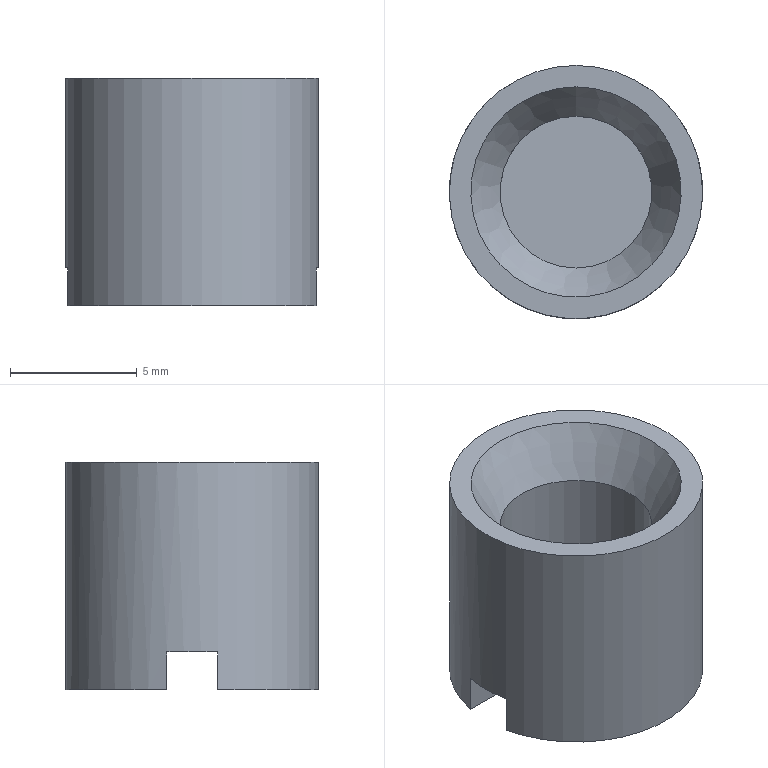Part | STEP file | 1-67.4 | 1 solid | 10 faces | box 10 x 10 x 9 mm | volume 482.855 mm3 | plane 7 | cylinder 2 | cone 1 | commonest cylinder face diameters 6 x1 10 x1
STEP:
#1=CARTESIAN_POINT('',(0.,0.,0.));
#2=DIRECTION('',(0.,0.,1.));
#3=DIRECTION('',(1.,0.,0.));
#4=AXIS2_PLACEMENT_3D('',#1,#2,#3);
#5=CARTESIAN_POINT('',(0.,5.,0.));
#6=VERTEX_POINT('',#5);
#7=CARTESIAN_POINT('',(-4.899,1.,0.));
#8=VERTEX_POINT('',#7);
#9=CARTESIAN_POINT('',(0.,0.,0.));
#10=DIRECTION('',(0.,0.,1.));
#11=DIRECTION('',(0.,1.,0.));
#12=AXIS2_PLACEMENT_3D('',#9,#10,#11);
#13=CIRCLE('',#12,5.);
#14=CARTESIAN_POINT('',(0.,-2.5,0.));
#15=DIRECTION('',(0.,0.,1.));
#16=DIRECTION('',(0.,1.,0.));
#17=AXIS2_PLACEMENT_3D('',#14,#15,#16);
#18=PLANE('',#17);
#19=CARTESIAN_POINT('',(2.5,0.));
#20=DIRECTION('',(1.,0.));
#21=AXIS2_PLACEMENT_2D('',#19,#20);
#22=CIRCLE('',#21,5.);
#23=(GEOMETRIC_REPRESENTATION_CONTEXT(2)PARAMETRIC_REPRESENTATION_CONTEXT()REPRESENTATION_CONTEXT('',''));
#24=DEFINITIONAL_REPRESENTATION('',(#22),#23);
#25=PCURVE('',#18,#24);
#26=CARTESIAN_POINT('',(0.,0.,0.));
#27=DIRECTION('',(0.,0.,1.));
#28=DIRECTION('',(0.,1.,0.));
#29=AXIS2_PLACEMENT_3D('',#26,#27,#28);
#30=CYLINDRICAL_SURFACE('',#29,5.);
#31=CARTESIAN_POINT('',(0.,0.));
#32=DIRECTION('',(1.,0.));
#33=VECTOR('',#32,1.);
#34=LINE('',#31,#33);
#35=(GEOMETRIC_REPRESENTATION_CONTEXT(2)PARAMETRIC_REPRESENTATION_CONTEXT()REPRESENTATION_CONTEXT('',''));
#36=DEFINITIONAL_REPRESENTATION('',(#34),#35);
#37=PCURVE('',#30,#36);
#38=SURFACE_CURVE('',#13,(#25,#37),.PCURVE_S1.);
#39=EDGE_CURVE('',#6,#8,#38,.T.);
#40=ORIENTED_EDGE('',*,*,#39,.T.);
#41=CARTESIAN_POINT('',(4.899,1.,0.));
#42=VERTEX_POINT('',#41);
#43=CARTESIAN_POINT('',(-4.899,1.,0.));
#44=DIRECTION('',(1.,0.,0.));
#45=VECTOR('',#44,1.);
#46=LINE('',#43,#45);
#47=CARTESIAN_POINT('',(3.5,4.899));
#48=DIRECTION('',(0.,-1.));
#49=VECTOR('',#48,1.);
#50=LINE('',#47,#49);
#51=(GEOMETRIC_REPRESENTATION_CONTEXT(2)PARAMETRIC_REPRESENTATION_CONTEXT()REPRESENTATION_CONTEXT('',''));
#52=DEFINITIONAL_REPRESENTATION('',(#50),#51);
#53=PCURVE('',#18,#52);
#54=CARTESIAN_POINT('',(0.,1.,0.));
#55=DIRECTION('',(0.,1.,0.));
#56=DIRECTION('',(0.,0.,1.));
#57=AXIS2_PLACEMENT_3D('',#54,#55,#56);
#58=PLANE('',#57);
#59=CARTESIAN_POINT('',(0.,-4.899));
#60=DIRECTION('',(0.,1.));
#61=VECTOR('',#60,1.);
#62=LINE('',#59,#61);
#63=(GEOMETRIC_REPRESENTATION_CONTEXT(2)PARAMETRIC_REPRESENTATION_CONTEXT()REPRESENTATION_CONTEXT('',''));
#64=DEFINITIONAL_REPRESENTATION('',(#62),#63);
#65=PCURVE('',#58,#64);
#66=SURFACE_CURVE('',#46,(#53,#65),.PCURVE_S1.);
#67=EDGE_CURVE('',#8,#42,#66,.T.);
#68=ORIENTED_EDGE('',*,*,#67,.T.);
#69=CARTESIAN_POINT('',(0.,0.,0.));
#70=DIRECTION('',(0.,0.,1.));
#71=DIRECTION('',(0.9798,0.2,0.));
#72=AXIS2_PLACEMENT_3D('',#69,#70,#71);
#73=CIRCLE('',#72,5.);
#74=CARTESIAN_POINT('',(2.5,0.));
#75=DIRECTION('',(0.2,-0.9798));
#76=AXIS2_PLACEMENT_2D('',#74,#75);
#77=CIRCLE('',#76,5.);
#78=(GEOMETRIC_REPRESENTATION_CONTEXT(2)PARAMETRIC_REPRESENTATION_CONTEXT()REPRESENTATION_CONTEXT('',''));
#79=DEFINITIONAL_REPRESENTATION('',(#77),#78);
#80=PCURVE('',#18,#79);
#81=CARTESIAN_POINT('',(4.914,0.));
#82=DIRECTION('',(1.,0.));
#83=VECTOR('',#82,1.);
#84=LINE('',#81,#83);
#85=(GEOMETRIC_REPRESENTATION_CONTEXT(2)PARAMETRIC_REPRESENTATION_CONTEXT()REPRESENTATION_CONTEXT('',''));
#86=DEFINITIONAL_REPRESENTATION('',(#84),#85);
#87=PCURVE('',#30,#86);
#88=SURFACE_CURVE('',#73,(#80,#87),.PCURVE_S1.);
#89=EDGE_CURVE('',#42,#6,#88,.T.);
#90=ORIENTED_EDGE('',*,*,#89,.T.);
#91=EDGE_LOOP('',(#40,#68,#90));
#92=FACE_BOUND('',#91,.F.);
#93=ADVANCED_FACE('',(#92),#18,.F.);
#94=CARTESIAN_POINT('',(-4.899,-1.,0.));
#95=VERTEX_POINT('',#94);
#96=CARTESIAN_POINT('',(4.899,-1.,0.));
#97=VERTEX_POINT('',#96);
#98=CARTESIAN_POINT('',(0.,0.,0.));
#99=DIRECTION('',(0.,0.,1.));
#100=DIRECTION('',(-0.9798,-0.2,0.));
#101=AXIS2_PLACEMENT_3D('',#98,#99,#100);
#102=CIRCLE('',#101,5.);
#103=CARTESIAN_POINT('',(0.,-2.5,0.));
#104=DIRECTION('',(0.,0.,1.));
#105=DIRECTION('',(0.,1.,0.));
#106=AXIS2_PLACEMENT_3D('',#103,#104,#105);
#107=PLANE('',#106);
#108=CARTESIAN_POINT('',(2.5,0.));
#109=DIRECTION('',(-0.2,0.9798));
#110=AXIS2_PLACEMENT_2D('',#108,#109);
#111=CIRCLE('',#110,5.);
#112=(GEOMETRIC_REPRESENTATION_CONTEXT(2)PARAMETRIC_REPRESENTATION_CONTEXT()REPRESENTATION_CONTEXT('',''));
#113=DEFINITIONAL_REPRESENTATION('',(#111),#112);
#114=PCURVE('',#107,#113);
#115=CARTESIAN_POINT('',(1.772,0.));
#116=DIRECTION('',(1.,0.));
#117=VECTOR('',#116,1.);
#118=LINE('',#115,#117);
#119=(GEOMETRIC_REPRESENTATION_CONTEXT(2)PARAMETRIC_REPRESENTATION_CONTEXT()REPRESENTATION_CONTEXT('',''));
#120=DEFINITIONAL_REPRESENTATION('',(#118),#119);
#121=PCURVE('',#30,#120);
#122=SURFACE_CURVE('',#102,(#114,#121),.PCURVE_S1.);
#123=EDGE_CURVE('',#95,#97,#122,.T.);
#124=ORIENTED_EDGE('',*,*,#123,.T.);
#125=CARTESIAN_POINT('',(4.899,-1.,0.));
#126=DIRECTION('',(-1.,0.,0.));
#127=VECTOR('',#126,1.);
#128=LINE('',#125,#127);
#129=CARTESIAN_POINT('',(1.5,-4.899));
#130=DIRECTION('',(0.,1.));
#131=VECTOR('',#130,1.);
#132=LINE('',#129,#131);
#133=(GEOMETRIC_REPRESENTATION_CONTEXT(2)PARAMETRIC_REPRESENTATION_CONTEXT()REPRESENTATION_CONTEXT('',''));
#134=DEFINITIONAL_REPRESENTATION('',(#132),#133);
#135=PCURVE('',#107,#134);
#136=CARTESIAN_POINT('',(0.,-1.,0.));
#137=DIRECTION('',(0.,-1.,0.));
#138=DIRECTION('',(0.,0.,-1.));
#139=AXIS2_PLACEMENT_3D('',#136,#137,#138);
#140=PLANE('',#139);
#141=CARTESIAN_POINT('',(0.,4.899));
#142=DIRECTION('',(0.,-1.));
#143=VECTOR('',#142,1.);
#144=LINE('',#141,#143);
#145=(GEOMETRIC_REPRESENTATION_CONTEXT(2)PARAMETRIC_REPRESENTATION_CONTEXT()REPRESENTATION_CONTEXT('',''));
#146=DEFINITIONAL_REPRESENTATION('',(#144),#145);
#147=PCURVE('',#140,#146);
#148=SURFACE_CURVE('',#128,(#135,#147),.PCURVE_S1.);
#149=EDGE_CURVE('',#97,#95,#148,.T.);
#150=ORIENTED_EDGE('',*,*,#149,.T.);
#151=EDGE_LOOP('',(#124,#150));
#152=FACE_BOUND('',#151,.F.);
#153=ADVANCED_FACE('',(#152),#107,.F.);
#154=ORIENTED_EDGE('',*,*,#39,.T.);
#155=CARTESIAN_POINT('',(-4.899,1.,1.5));
#156=VERTEX_POINT('',#155);
#157=CARTESIAN_POINT('',(-4.899,1.,1.5));
#158=DIRECTION('',(0.,0.,-1.));
#159=VECTOR('',#158,1.);
#160=LINE('',#157,#159);
#161=CARTESIAN_POINT('',(1.369,1.5));
#162=DIRECTION('',(0.,-1.));
#163=VECTOR('',#162,1.);
#164=LINE('',#161,#163);
#165=(GEOMETRIC_REPRESENTATION_CONTEXT(2)PARAMETRIC_REPRESENTATION_CONTEXT()REPRESENTATION_CONTEXT('',''));
#166=DEFINITIONAL_REPRESENTATION('',(#164),#165);
#167=PCURVE('',#30,#166);
#168=CARTESIAN_POINT('',(1.5,-4.899));
#169=DIRECTION('',(-1.,0.));
#170=VECTOR('',#169,1.);
#171=LINE('',#168,#170);
#172=(GEOMETRIC_REPRESENTATION_CONTEXT(2)PARAMETRIC_REPRESENTATION_CONTEXT()REPRESENTATION_CONTEXT('',''));
#173=DEFINITIONAL_REPRESENTATION('',(#171),#172);
#174=PCURVE('',#58,#173);
#175=SURFACE_CURVE('',#160,(#167,#174),.PCURVE_S1.);
#176=EDGE_CURVE('',#156,#8,#175,.T.);
#177=ORIENTED_EDGE('',*,*,#176,.F.);
#178=CARTESIAN_POINT('',(-4.899,-1.,1.5));
#179=VERTEX_POINT('',#178);
#180=CARTESIAN_POINT('',(0.,0.,1.5));
#181=DIRECTION('',(0.,0.,-1.));
#182=DIRECTION('',(-0.9798,-0.2,0.));
#183=AXIS2_PLACEMENT_3D('',#180,#181,#182);
#184=CIRCLE('',#183,5.);
#185=CARTESIAN_POINT('',(1.772,1.5));
#186=DIRECTION('',(-1.,0.));
#187=VECTOR('',#186,1.);
#188=LINE('',#185,#187);
#189=(GEOMETRIC_REPRESENTATION_CONTEXT(2)PARAMETRIC_REPRESENTATION_CONTEXT()REPRESENTATION_CONTEXT('',''));
#190=DEFINITIONAL_REPRESENTATION('',(#188),#189);
#191=PCURVE('',#30,#190);
#192=CARTESIAN_POINT('',(0.,0.,1.5));
#193=DIRECTION('',(0.,0.,1.));
#194=DIRECTION('',(0.,-1.,0.));
#195=AXIS2_PLACEMENT_3D('',#192,#193,#194);
#196=PLANE('',#195);
#197=CARTESIAN_POINT('',(1.,-4.899));
#198=CARTESIAN_POINT('',(-7.485,-6.631));
#199=CARTESIAN_POINT('',(-4.743,1.583));
#200=CARTESIAN_POINT('',(-2.,9.798));
#201=CARTESIAN_POINT('',(3.743,3.316));
#202=CARTESIAN_POINT('',(9.485,-3.167));
#203=CARTESIAN_POINT('',(1.,-4.899));
#204=(BOUNDED_CURVE()B_SPLINE_CURVE(2,(#197,#198,#199,#200,#201,#202,#203),.UNSPECIFIED.,.T.,.F.)B_SPLINE_CURVE_WITH_KNOTS((1,2,2,2,2,1),(-2.094,0.,2.094,4.189,6.283,8.378),.UNSPECIFIED.)CURVE()GEOMETRIC_REPRESENTATION_ITEM()RATIONAL_B_SPLINE_CURVE((1.,0.5,1.,0.5,1.,0.5,1.))REPRESENTATION_ITEM(''));
#205=(GEOMETRIC_REPRESENTATION_CONTEXT(2)PARAMETRIC_REPRESENTATION_CONTEXT()REPRESENTATION_CONTEXT('',''));
#206=DEFINITIONAL_REPRESENTATION('',(#204),#205);
#207=PCURVE('',#196,#206);
#208=SURFACE_CURVE('',#184,(#191,#207),.PCURVE_S1.);
#209=EDGE_CURVE('',#179,#156,#208,.T.);
#210=ORIENTED_EDGE('',*,*,#209,.F.);
#211=CARTESIAN_POINT('',(-4.899,-1.,0.));
#212=DIRECTION('',(0.,0.,1.));
#213=VECTOR('',#212,1.);
#214=LINE('',#211,#213);
#215=CARTESIAN_POINT('',(1.772,0.));
#216=DIRECTION('',(0.,1.));
#217=VECTOR('',#216,1.);
#218=LINE('',#215,#217);
#219=(GEOMETRIC_REPRESENTATION_CONTEXT(2)PARAMETRIC_REPRESENTATION_CONTEXT()REPRESENTATION_CONTEXT('',''));
#220=DEFINITIONAL_REPRESENTATION('',(#218),#219);
#221=PCURVE('',#30,#220);
#222=CARTESIAN_POINT('',(0.,-4.899));
#223=DIRECTION('',(-1.,0.));
#224=VECTOR('',#223,1.);
#225=LINE('',#222,#224);
#226=(GEOMETRIC_REPRESENTATION_CONTEXT(2)PARAMETRIC_REPRESENTATION_CONTEXT()REPRESENTATION_CONTEXT('',''));
#227=DEFINITIONAL_REPRESENTATION('',(#225),#226);
#228=PCURVE('',#140,#227);
#229=SURFACE_CURVE('',#214,(#221,#228),.PCURVE_S1.);
#230=EDGE_CURVE('',#95,#179,#229,.T.);
#231=ORIENTED_EDGE('',*,*,#230,.F.);
#232=ORIENTED_EDGE('',*,*,#123,.T.);
#233=CARTESIAN_POINT('',(4.899,-1.,1.5));
#234=VERTEX_POINT('',#233);
#235=CARTESIAN_POINT('',(4.899,-1.,1.5));
#236=DIRECTION('',(0.,0.,-1.));
#237=VECTOR('',#236,1.);
#238=LINE('',#235,#237);
#239=CARTESIAN_POINT('',(4.511,1.5));
#240=DIRECTION('',(0.,-1.));
#241=VECTOR('',#240,1.);
#242=LINE('',#239,#241);
#243=(GEOMETRIC_REPRESENTATION_CONTEXT(2)PARAMETRIC_REPRESENTATION_CONTEXT()REPRESENTATION_CONTEXT('',''));
#244=DEFINITIONAL_REPRESENTATION('',(#242),#243);
#245=PCURVE('',#30,#244);
#246=CARTESIAN_POINT('',(-1.5,4.899));
#247=DIRECTION('',(1.,0.));
#248=VECTOR('',#247,1.);
#249=LINE('',#246,#248);
#250=(GEOMETRIC_REPRESENTATION_CONTEXT(2)PARAMETRIC_REPRESENTATION_CONTEXT()REPRESENTATION_CONTEXT('',''));
#251=DEFINITIONAL_REPRESENTATION('',(#249),#250);
#252=PCURVE('',#140,#251);
#253=SURFACE_CURVE('',#238,(#245,#252),.PCURVE_S1.);
#254=EDGE_CURVE('',#234,#97,#253,.T.);
#255=ORIENTED_EDGE('',*,*,#254,.F.);
#256=CARTESIAN_POINT('',(4.899,1.,1.5));
#257=VERTEX_POINT('',#256);
#258=CARTESIAN_POINT('',(0.,0.,1.5));
#259=DIRECTION('',(0.,0.,-1.));
#260=DIRECTION('',(0.9798,0.2,0.));
#261=AXIS2_PLACEMENT_3D('',#258,#259,#260);
#262=CIRCLE('',#261,5.);
#263=CARTESIAN_POINT('',(4.914,1.5));
#264=DIRECTION('',(-1.,0.));
#265=VECTOR('',#264,1.);
#266=LINE('',#263,#265);
#267=(GEOMETRIC_REPRESENTATION_CONTEXT(2)PARAMETRIC_REPRESENTATION_CONTEXT()REPRESENTATION_CONTEXT('',''));
#268=DEFINITIONAL_REPRESENTATION('',(#266),#267);
#269=PCURVE('',#30,#268);
#270=CARTESIAN_POINT('',(-1.,4.899));
#271=CARTESIAN_POINT('',(7.485,6.631));
#272=CARTESIAN_POINT('',(4.743,-1.583));
#273=CARTESIAN_POINT('',(2.,-9.798));
#274=CARTESIAN_POINT('',(-3.743,-3.316));
#275=CARTESIAN_POINT('',(-9.485,3.167));
#276=CARTESIAN_POINT('',(-1.,4.899));
#277=(BOUNDED_CURVE()B_SPLINE_CURVE(2,(#270,#271,#272,#273,#274,#275,#276),.UNSPECIFIED.,.T.,.F.)B_SPLINE_CURVE_WITH_KNOTS((1,2,2,2,2,1),(-2.094,0.,2.094,4.189,6.283,8.378),.UNSPECIFIED.)CURVE()GEOMETRIC_REPRESENTATION_ITEM()RATIONAL_B_SPLINE_CURVE((1.,0.5,1.,0.5,1.,0.5,1.))REPRESENTATION_ITEM(''));
#278=(GEOMETRIC_REPRESENTATION_CONTEXT(2)PARAMETRIC_REPRESENTATION_CONTEXT()REPRESENTATION_CONTEXT('',''));
#279=DEFINITIONAL_REPRESENTATION('',(#277),#278);
#280=PCURVE('',#196,#279);
#281=SURFACE_CURVE('',#262,(#269,#280),.PCURVE_S1.);
#282=EDGE_CURVE('',#257,#234,#281,.T.);
#283=ORIENTED_EDGE('',*,*,#282,.F.);
#284=CARTESIAN_POINT('',(4.899,1.,0.));
#285=DIRECTION('',(0.,0.,1.));
#286=VECTOR('',#285,1.);
#287=LINE('',#284,#286);
#288=CARTESIAN_POINT('',(4.914,0.));
#289=DIRECTION('',(0.,1.));
#290=VECTOR('',#289,1.);
#291=LINE('',#288,#290);
#292=(GEOMETRIC_REPRESENTATION_CONTEXT(2)PARAMETRIC_REPRESENTATION_CONTEXT()REPRESENTATION_CONTEXT('',''));
#293=DEFINITIONAL_REPRESENTATION('',(#291),#292);
#294=PCURVE('',#30,#293);
#295=CARTESIAN_POINT('',(0.,4.899));
#296=DIRECTION('',(1.,0.));
#297=VECTOR('',#296,1.);
#298=LINE('',#295,#297);
#299=(GEOMETRIC_REPRESENTATION_CONTEXT(2)PARAMETRIC_REPRESENTATION_CONTEXT()REPRESENTATION_CONTEXT('',''));
#300=DEFINITIONAL_REPRESENTATION('',(#298),#299);
#301=PCURVE('',#58,#300);
#302=SURFACE_CURVE('',#287,(#294,#301),.PCURVE_S1.);
#303=EDGE_CURVE('',#42,#257,#302,.T.);
#304=ORIENTED_EDGE('',*,*,#303,.F.);
#305=ORIENTED_EDGE('',*,*,#89,.T.);
#306=CARTESIAN_POINT('',(0.,5.,9.));
#307=VERTEX_POINT('',#306);
#308=CARTESIAN_POINT('',(0.,5.,0.));
#309=DIRECTION('',(0.,0.,1.));
#310=VECTOR('',#309,1.);
#311=LINE('',#308,#310);
#312=CARTESIAN_POINT('',(6.283,0.));
#313=DIRECTION('',(0.,1.));
#314=VECTOR('',#313,1.);
#315=LINE('',#312,#314);
#316=(GEOMETRIC_REPRESENTATION_CONTEXT(2)PARAMETRIC_REPRESENTATION_CONTEXT()REPRESENTATION_CONTEXT('',''));
#317=DEFINITIONAL_REPRESENTATION('',(#315),#316);
#318=PCURVE('',#30,#317);
#319=CARTESIAN_POINT('',(0.,0.));
#320=DIRECTION('',(0.,1.));
#321=VECTOR('',#320,1.);
#322=LINE('',#319,#321);
#323=(GEOMETRIC_REPRESENTATION_CONTEXT(2)PARAMETRIC_REPRESENTATION_CONTEXT()REPRESENTATION_CONTEXT('',''));
#324=DEFINITIONAL_REPRESENTATION('',(#322),#323);
#325=PCURVE('',#30,#324);
#326=SEAM_CURVE('',#311,(#318,#325),.PCURVE_S1.);
#327=EDGE_CURVE('',#6,#307,#326,.T.);
#328=ORIENTED_EDGE('',*,*,#327,.T.);
#329=CARTESIAN_POINT('',(0.,0.,9.));
#330=DIRECTION('',(0.,0.,1.));
#331=DIRECTION('',(0.,1.,0.));
#332=AXIS2_PLACEMENT_3D('',#329,#330,#331);
#333=CIRCLE('',#332,5.);
#334=CARTESIAN_POINT('',(0.,9.));
#335=DIRECTION('',(1.,0.));
#336=VECTOR('',#335,1.);
#337=LINE('',#334,#336);
#338=(GEOMETRIC_REPRESENTATION_CONTEXT(2)PARAMETRIC_REPRESENTATION_CONTEXT()REPRESENTATION_CONTEXT('',''));
#339=DEFINITIONAL_REPRESENTATION('',(#337),#338);
#340=PCURVE('',#30,#339);
#341=CARTESIAN_POINT('',(0.,-1.34,9.));
#342=DIRECTION('',(0.,0.,1.));
#343=DIRECTION('',(0.,1.,0.));
#344=AXIS2_PLACEMENT_3D('',#341,#342,#343);
#345=PLANE('',#344);
#346=CARTESIAN_POINT('',(1.34,0.));
#347=DIRECTION('',(1.,0.));
#348=AXIS2_PLACEMENT_2D('',#346,#347);
#349=CIRCLE('',#348,5.);
#350=(GEOMETRIC_REPRESENTATION_CONTEXT(2)PARAMETRIC_REPRESENTATION_CONTEXT()REPRESENTATION_CONTEXT('',''));
#351=DEFINITIONAL_REPRESENTATION('',(#349),#350);
#352=PCURVE('',#345,#351);
#353=SURFACE_CURVE('',#333,(#340,#352),.PCURVE_S1.);
#354=EDGE_CURVE('',#307,#307,#353,.T.);
#355=ORIENTED_EDGE('',*,*,#354,.F.);
#356=ORIENTED_EDGE('',*,*,#327,.F.);
#357=EDGE_LOOP('',(#154,#177,#210,#231,#232,#255,#283,#304,#305,#328,#355,#356));
#358=FACE_BOUND('',#357,.T.);
#359=ADVANCED_FACE('',(#358),#30,.T.);
#360=CARTESIAN_POINT('',(-4.899,1.,1.5));
#361=DIRECTION('',(1.,0.,0.));
#362=VECTOR('',#361,1.);
#363=LINE('',#360,#362);
#364=CARTESIAN_POINT('',(1.5,-4.899));
#365=DIRECTION('',(0.,1.));
#366=VECTOR('',#365,1.);
#367=LINE('',#364,#366);
#368=(GEOMETRIC_REPRESENTATION_CONTEXT(2)PARAMETRIC_REPRESENTATION_CONTEXT()REPRESENTATION_CONTEXT('',''));
#369=DEFINITIONAL_REPRESENTATION('',(#367),#368);
#370=PCURVE('',#58,#369);
#371=CARTESIAN_POINT('',(-1.,-4.899));
#372=DIRECTION('',(0.,1.));
#373=VECTOR('',#372,1.);
#374=LINE('',#371,#373);
#375=(GEOMETRIC_REPRESENTATION_CONTEXT(2)PARAMETRIC_REPRESENTATION_CONTEXT()REPRESENTATION_CONTEXT('',''));
#376=DEFINITIONAL_REPRESENTATION('',(#374),#375);
#377=PCURVE('',#196,#376);
#378=SURFACE_CURVE('',#363,(#370,#377),.PCURVE_S1.);
#379=EDGE_CURVE('',#156,#257,#378,.T.);
#380=ORIENTED_EDGE('',*,*,#379,.T.);
#381=ORIENTED_EDGE('',*,*,#303,.F.);
#382=ORIENTED_EDGE('',*,*,#67,.F.);
#383=ORIENTED_EDGE('',*,*,#176,.F.);
#384=EDGE_LOOP('',(#380,#381,#382,#383));
#385=FACE_BOUND('',#384,.F.);
#386=ADVANCED_FACE('',(#385),#58,.F.);
#387=ORIENTED_EDGE('',*,*,#379,.F.);
#388=ORIENTED_EDGE('',*,*,#209,.F.);
#389=CARTESIAN_POINT('',(-4.899,-1.,1.5));
#390=DIRECTION('',(1.,0.,0.));
#391=VECTOR('',#390,1.);
#392=LINE('',#389,#391);
#393=CARTESIAN_POINT('',(1.,-4.899));
#394=DIRECTION('',(0.,1.));
#395=VECTOR('',#394,1.);
#396=LINE('',#393,#395);
#397=(GEOMETRIC_REPRESENTATION_CONTEXT(2)PARAMETRIC_REPRESENTATION_CONTEXT()REPRESENTATION_CONTEXT('',''));
#398=DEFINITIONAL_REPRESENTATION('',(#396),#397);
#399=PCURVE('',#196,#398);
#400=CARTESIAN_POINT('',(-1.5,-4.899));
#401=DIRECTION('',(0.,1.));
#402=VECTOR('',#401,1.);
#403=LINE('',#400,#402);
#404=(GEOMETRIC_REPRESENTATION_CONTEXT(2)PARAMETRIC_REPRESENTATION_CONTEXT()REPRESENTATION_CONTEXT('',''));
#405=DEFINITIONAL_REPRESENTATION('',(#403),#404);
#406=PCURVE('',#140,#405);
#407=SURFACE_CURVE('',#392,(#399,#406),.PCURVE_S1.);
#408=EDGE_CURVE('',#179,#234,#407,.T.);
#409=ORIENTED_EDGE('',*,*,#408,.T.);
#410=ORIENTED_EDGE('',*,*,#282,.F.);
#411=EDGE_LOOP('',(#387,#388,#409,#410));
#412=FACE_BOUND('',#411,.F.);
#413=ADVANCED_FACE('',(#412),#196,.F.);
#414=ORIENTED_EDGE('',*,*,#408,.F.);
#415=ORIENTED_EDGE('',*,*,#230,.F.);
#416=ORIENTED_EDGE('',*,*,#149,.F.);
#417=ORIENTED_EDGE('',*,*,#254,.F.);
#418=EDGE_LOOP('',(#414,#415,#416,#417));
#419=FACE_BOUND('',#418,.F.);
#420=ADVANCED_FACE('',(#419),#140,.F.);
#421=ORIENTED_EDGE('',*,*,#354,.T.);
#422=EDGE_LOOP('',(#421));
#423=FACE_BOUND('',#422,.T.);
#424=CARTESIAN_POINT('',(0.,4.155,9.));
#425=VERTEX_POINT('',#424);
#426=CARTESIAN_POINT('',(0.,0.,9.));
#427=DIRECTION('',(0.,0.,-1.));
#428=DIRECTION('',(0.,1.,0.));
#429=AXIS2_PLACEMENT_3D('',#426,#427,#428);
#430=CIRCLE('',#429,4.155);
#431=CARTESIAN_POINT('',(5.494,0.));
#432=CARTESIAN_POINT('',(5.494,-7.196));
#433=CARTESIAN_POINT('',(-0.7376,-3.598));
#434=CARTESIAN_POINT('',(-6.97,0.));
#435=CARTESIAN_POINT('',(-0.7376,3.598));
#436=CARTESIAN_POINT('',(5.494,7.196));
#437=CARTESIAN_POINT('',(5.494,0.));
#438=(BOUNDED_CURVE()B_SPLINE_CURVE(2,(#431,#432,#433,#434,#435,#436,#437),.UNSPECIFIED.,.T.,.F.)B_SPLINE_CURVE_WITH_KNOTS((1,2,2,2,2,1),(-2.094,0.,2.094,4.189,6.283,8.378),.UNSPECIFIED.)CURVE()GEOMETRIC_REPRESENTATION_ITEM()RATIONAL_B_SPLINE_CURVE((1.,0.5,1.,0.5,1.,0.5,1.))REPRESENTATION_ITEM(''));
#439=(GEOMETRIC_REPRESENTATION_CONTEXT(2)PARAMETRIC_REPRESENTATION_CONTEXT()REPRESENTATION_CONTEXT('',''));
#440=DEFINITIONAL_REPRESENTATION('',(#438),#439);
#441=PCURVE('',#345,#440);
#442=CARTESIAN_POINT('',(0.,0.,7.));
#443=DIRECTION('',(0.,0.,1.));
#444=DIRECTION('',(0.,1.,0.));
#445=AXIS2_PLACEMENT_3D('',#442,#443,#444);
#446=CONICAL_SURFACE('',#445,3.,0.5236);
#447=CARTESIAN_POINT('',(6.283,2.));
#448=DIRECTION('',(-1.,0.));
#449=VECTOR('',#448,1.);
#450=LINE('',#447,#449);
#451=(GEOMETRIC_REPRESENTATION_CONTEXT(2)PARAMETRIC_REPRESENTATION_CONTEXT()REPRESENTATION_CONTEXT('',''));
#452=DEFINITIONAL_REPRESENTATION('',(#450),#451);
#453=PCURVE('',#446,#452);
#454=SURFACE_CURVE('',#430,(#441,#453),.PCURVE_S1.);
#455=EDGE_CURVE('',#425,#425,#454,.T.);
#456=ORIENTED_EDGE('',*,*,#455,.T.);
#457=EDGE_LOOP('',(#456));
#458=FACE_BOUND('',#457,.T.);
#459=ADVANCED_FACE('',(#423,#458),#345,.T.);
#460=CARTESIAN_POINT('',(0.,3.,7.));
#461=VERTEX_POINT('',#460);
#462=CARTESIAN_POINT('',(0.,3.,7.));
#463=DIRECTION('',(0.,0.5,0.866));
#464=VECTOR('',#463,1.);
#465=LINE('',#462,#464);
#466=CARTESIAN_POINT('',(6.283,0.));
#467=DIRECTION('',(0.,1.));
#468=VECTOR('',#467,1.);
#469=LINE('',#466,#468);
#470=(GEOMETRIC_REPRESENTATION_CONTEXT(2)PARAMETRIC_REPRESENTATION_CONTEXT()REPRESENTATION_CONTEXT('',''));
#471=DEFINITIONAL_REPRESENTATION('',(#469),#470);
#472=PCURVE('',#446,#471);
#473=CARTESIAN_POINT('',(0.,0.));
#474=DIRECTION('',(0.,1.));
#475=VECTOR('',#474,1.);
#476=LINE('',#473,#475);
#477=(GEOMETRIC_REPRESENTATION_CONTEXT(2)PARAMETRIC_REPRESENTATION_CONTEXT()REPRESENTATION_CONTEXT('',''));
#478=DEFINITIONAL_REPRESENTATION('',(#476),#477);
#479=PCURVE('',#446,#478);
#480=SEAM_CURVE('',#465,(#472,#479),.PCURVE_S1.);
#481=EDGE_CURVE('',#461,#425,#480,.T.);
#482=ORIENTED_EDGE('',*,*,#481,.T.);
#483=ORIENTED_EDGE('',*,*,#455,.T.);
#484=ORIENTED_EDGE('',*,*,#481,.F.);
#485=CARTESIAN_POINT('',(0.,0.,7.));
#486=DIRECTION('',(0.,0.,-1.));
#487=DIRECTION('',(0.,1.,0.));
#488=AXIS2_PLACEMENT_3D('',#485,#486,#487);
#489=CIRCLE('',#488,3.);
#490=CARTESIAN_POINT('',(6.283,0.));
#491=DIRECTION('',(-1.,0.));
#492=VECTOR('',#491,1.);
#493=LINE('',#490,#492);
#494=(GEOMETRIC_REPRESENTATION_CONTEXT(2)PARAMETRIC_REPRESENTATION_CONTEXT()REPRESENTATION_CONTEXT('',''));
#495=DEFINITIONAL_REPRESENTATION('',(#493),#494);
#496=PCURVE('',#446,#495);
#497=CARTESIAN_POINT('',(0.,0.,3.));
#498=DIRECTION('',(0.,0.,1.));
#499=DIRECTION('',(0.,1.,0.));
#500=AXIS2_PLACEMENT_3D('',#497,#498,#499);
#501=CYLINDRICAL_SURFACE('',#500,3.);
#502=CARTESIAN_POINT('',(6.283,4.));
#503=DIRECTION('',(-1.,0.));
#504=VECTOR('',#503,1.);
#505=LINE('',#502,#504);
#506=(GEOMETRIC_REPRESENTATION_CONTEXT(2)PARAMETRIC_REPRESENTATION_CONTEXT()REPRESENTATION_CONTEXT('',''));
#507=DEFINITIONAL_REPRESENTATION('',(#505),#506);
#508=PCURVE('',#501,#507);
#509=SURFACE_CURVE('',#489,(#496,#508),.PCURVE_S1.);
#510=EDGE_CURVE('',#461,#461,#509,.T.);
#511=ORIENTED_EDGE('',*,*,#510,.F.);
#512=EDGE_LOOP('',(#482,#483,#484,#511));
#513=FACE_BOUND('',#512,.F.);
#514=ADVANCED_FACE('',(#513),#446,.F.);
#515=CARTESIAN_POINT('',(0.,3.,3.));
#516=VERTEX_POINT('',#515);
#517=CARTESIAN_POINT('',(0.,3.,3.));
#518=DIRECTION('',(0.,0.,1.));
#519=VECTOR('',#518,1.);
#520=LINE('',#517,#519);
#521=CARTESIAN_POINT('',(6.283,0.));
#522=DIRECTION('',(0.,1.));
#523=VECTOR('',#522,1.);
#524=LINE('',#521,#523);
#525=(GEOMETRIC_REPRESENTATION_CONTEXT(2)PARAMETRIC_REPRESENTATION_CONTEXT()REPRESENTATION_CONTEXT('',''));
#526=DEFINITIONAL_REPRESENTATION('',(#524),#525);
#527=PCURVE('',#501,#526);
#528=CARTESIAN_POINT('',(0.,0.));
#529=DIRECTION('',(0.,1.));
#530=VECTOR('',#529,1.);
#531=LINE('',#528,#530);
#532=(GEOMETRIC_REPRESENTATION_CONTEXT(2)PARAMETRIC_REPRESENTATION_CONTEXT()REPRESENTATION_CONTEXT('',''));
#533=DEFINITIONAL_REPRESENTATION('',(#531),#532);
#534=PCURVE('',#501,#533);
#535=SEAM_CURVE('',#520,(#527,#534),.PCURVE_S1.);
#536=EDGE_CURVE('',#516,#461,#535,.T.);
#537=ORIENTED_EDGE('',*,*,#536,.T.);
#538=ORIENTED_EDGE('',*,*,#510,.T.);
#539=ORIENTED_EDGE('',*,*,#536,.F.);
#540=CARTESIAN_POINT('',(0.,0.,3.));
#541=DIRECTION('',(0.,0.,-1.));
#542=DIRECTION('',(0.,1.,0.));
#543=AXIS2_PLACEMENT_3D('',#540,#541,#542);
#544=CIRCLE('',#543,3.);
#545=CARTESIAN_POINT('',(6.283,0.));
#546=DIRECTION('',(-1.,0.));
#547=VECTOR('',#546,1.);
#548=LINE('',#545,#547);
#549=(GEOMETRIC_REPRESENTATION_CONTEXT(2)PARAMETRIC_REPRESENTATION_CONTEXT()REPRESENTATION_CONTEXT('',''));
#550=DEFINITIONAL_REPRESENTATION('',(#548),#549);
#551=PCURVE('',#501,#550);
#552=CARTESIAN_POINT('',(0.,0.,3.));
#553=DIRECTION('',(0.,0.,-1.));
#554=DIRECTION('',(0.,1.,0.));
#555=AXIS2_PLACEMENT_3D('',#552,#553,#554);
#556=PLANE('',#555);
#557=CARTESIAN_POINT('',(0.,0.));
#558=DIRECTION('',(1.,0.));
#559=AXIS2_PLACEMENT_2D('',#557,#558);
#560=CIRCLE('',#559,3.);
#561=(GEOMETRIC_REPRESENTATION_CONTEXT(2)PARAMETRIC_REPRESENTATION_CONTEXT()REPRESENTATION_CONTEXT('',''));
#562=DEFINITIONAL_REPRESENTATION('',(#560),#561);
#563=PCURVE('',#556,#562);
#564=SURFACE_CURVE('',#544,(#551,#563),.PCURVE_S1.);
#565=EDGE_CURVE('',#516,#516,#564,.T.);
#566=ORIENTED_EDGE('',*,*,#565,.F.);
#567=EDGE_LOOP('',(#537,#538,#539,#566));
#568=FACE_BOUND('',#567,.F.);
#569=ADVANCED_FACE('',(#568),#501,.F.);
#570=ORIENTED_EDGE('',*,*,#565,.T.);
#571=EDGE_LOOP('',(#570));
#572=FACE_BOUND('',#571,.F.);
#573=ADVANCED_FACE('',(#572),#556,.F.);
#574=CLOSED_SHELL('',(#93,#153,#359,#386,#413,#420,#459,#514,#569,#573));
#575=MANIFOLD_SOLID_BREP('',#574);
#576=(LENGTH_UNIT()NAMED_UNIT(*)SI_UNIT(.MILLI.,.METRE.));
#577=UNCERTAINTY_MEASURE_WITH_UNIT(LENGTH_MEASURE(0.0000001),#576,'','');
#578=(NAMED_UNIT(*)PLANE_ANGLE_UNIT()SI_UNIT($,.RADIAN.));
#579=(NAMED_UNIT(*)SI_UNIT($,.STERADIAN.)SOLID_ANGLE_UNIT());
#580=(GEOMETRIC_REPRESENTATION_CONTEXT(3)GLOBAL_UNCERTAINTY_ASSIGNED_CONTEXT((#577))GLOBAL_UNIT_ASSIGNED_CONTEXT((#576,#578,#579))REPRESENTATION_CONTEXT('',''));
#581=ADVANCED_BREP_SHAPE_REPRESENTATION('',(#4,#575),#580);